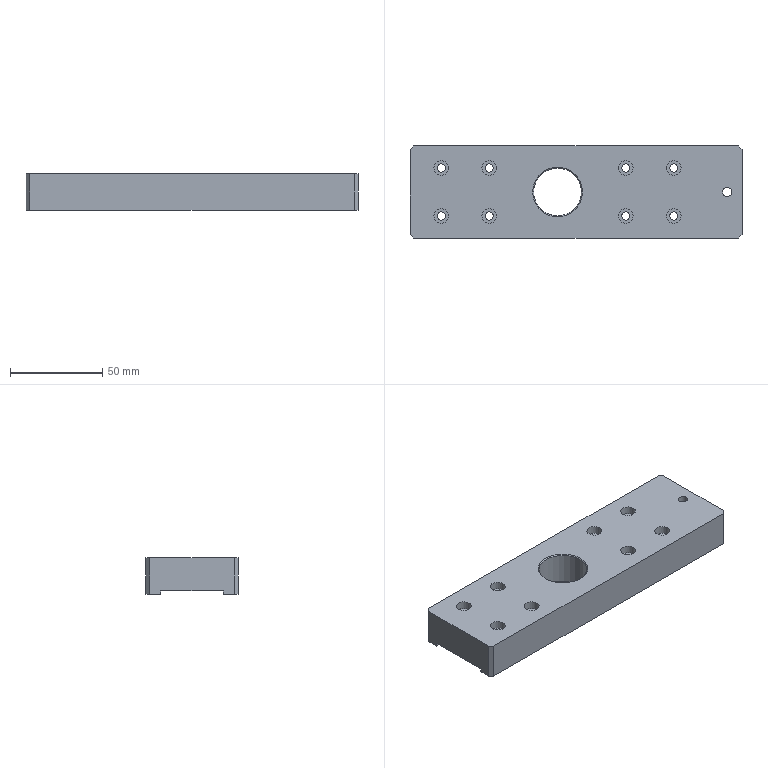Part | NX | 1 solid | 42 faces | box 180 x 50 x 20 mm | volume 154777 mm3 | plane 22 | cylinder 18 | cone 2 | commonest cylinder face diameters 4.5 x8 8 x8 5 x1 26 x1
STEP:
#1=CARTESIAN_POINT('',(-88.,25.,10.));
#2=VERTEX_POINT('',#1);
#3=CARTESIAN_POINT('',(-90.,23.,10.));
#4=VERTEX_POINT('',#3);
#5=CARTESIAN_POINT('',(-56.5,56.5,10.));
#6=DIRECTION('',(-0.7071,-0.7071,0.));
#7=VECTOR('',#6,1000.);
#8=LINE('',#5,#7);
#9=EDGE_CURVE('',#2,#4,#8,.T.);
#10=ORIENTED_EDGE('',*,*,#9,.F.);
#11=CARTESIAN_POINT('',(-88.,25.,-10.));
#12=VERTEX_POINT('',#11);
#13=CARTESIAN_POINT('',(-88.,25.,10.));
#14=DIRECTION('',(0.,0.,1.));
#15=VECTOR('',#14,1000.);
#16=LINE('',#13,#15);
#17=EDGE_CURVE('',#12,#2,#16,.T.);
#18=ORIENTED_EDGE('',*,*,#17,.F.);
#19=CARTESIAN_POINT('',(-90.,23.,-10.));
#20=VERTEX_POINT('',#19);
#21=CARTESIAN_POINT('',(-90.,23.,-10.));
#22=DIRECTION('',(0.7071,0.7071,0.));
#23=VECTOR('',#22,1000.);
#24=LINE('',#21,#23);
#25=EDGE_CURVE('',#20,#12,#24,.T.);
#26=ORIENTED_EDGE('',*,*,#25,.F.);
#27=CARTESIAN_POINT('',(-90.,23.,10.));
#28=DIRECTION('',(0.,0.,-1.));
#29=VECTOR('',#28,1000.);
#30=LINE('',#27,#29);
#31=EDGE_CURVE('',#4,#20,#30,.T.);
#32=ORIENTED_EDGE('',*,*,#31,.F.);
#33=EDGE_LOOP('',(#10,#18,#26,#32));
#34=FACE_BOUND('',#33,.T.);
#35=CARTESIAN_POINT('',(-90.,23.,10.));
#36=DIRECTION('',(0.7071,-0.7071,0.));
#37=DIRECTION('',(0.,0.,-1.));
#38=AXIS2_PLACEMENT_3D('',#35,#36,#37);
#39=PLANE('',#38);
#40=ADVANCED_FACE('',(#34),#39,.F.);
#41=CARTESIAN_POINT('',(-90.,-23.,10.));
#42=VERTEX_POINT('',#41);
#43=CARTESIAN_POINT('',(-88.,-25.,10.));
#44=VERTEX_POINT('',#43);
#45=CARTESIAN_POINT('',(-56.5,-56.5,10.));
#46=DIRECTION('',(0.7071,-0.7071,0.));
#47=VECTOR('',#46,1000.);
#48=LINE('',#45,#47);
#49=EDGE_CURVE('',#42,#44,#48,.T.);
#50=ORIENTED_EDGE('',*,*,#49,.F.);
#51=CARTESIAN_POINT('',(-90.,-23.,-10.));
#52=VERTEX_POINT('',#51);
#53=CARTESIAN_POINT('',(-90.,-23.,10.));
#54=DIRECTION('',(0.,0.,1.));
#55=VECTOR('',#54,1000.);
#56=LINE('',#53,#55);
#57=EDGE_CURVE('',#52,#42,#56,.T.);
#58=ORIENTED_EDGE('',*,*,#57,.F.);
#59=CARTESIAN_POINT('',(-88.,-25.,-10.));
#60=VERTEX_POINT('',#59);
#61=CARTESIAN_POINT('',(-88.,-25.,-10.));
#62=DIRECTION('',(-0.7071,0.7071,0.));
#63=VECTOR('',#62,1000.);
#64=LINE('',#61,#63);
#65=EDGE_CURVE('',#60,#52,#64,.T.);
#66=ORIENTED_EDGE('',*,*,#65,.F.);
#67=CARTESIAN_POINT('',(-88.,-25.,10.));
#68=DIRECTION('',(0.,0.,-1.));
#69=VECTOR('',#68,1000.);
#70=LINE('',#67,#69);
#71=EDGE_CURVE('',#44,#60,#70,.T.);
#72=ORIENTED_EDGE('',*,*,#71,.F.);
#73=EDGE_LOOP('',(#50,#58,#66,#72));
#74=FACE_BOUND('',#73,.T.);
#75=CARTESIAN_POINT('',(-88.,-25.,10.));
#76=DIRECTION('',(0.7071,0.7071,0.));
#77=DIRECTION('',(0.,0.,-1.));
#78=AXIS2_PLACEMENT_3D('',#75,#76,#77);
#79=PLANE('',#78);
#80=ADVANCED_FACE('',(#74),#79,.F.);
#81=CARTESIAN_POINT('',(88.,-25.,10.));
#82=VERTEX_POINT('',#81);
#83=CARTESIAN_POINT('',(90.,-23.,10.));
#84=VERTEX_POINT('',#83);
#85=CARTESIAN_POINT('',(56.5,-56.5,10.));
#86=DIRECTION('',(0.7071,0.7071,0.));
#87=VECTOR('',#86,1000.);
#88=LINE('',#85,#87);
#89=EDGE_CURVE('',#82,#84,#88,.T.);
#90=ORIENTED_EDGE('',*,*,#89,.F.);
#91=CARTESIAN_POINT('',(88.,-25.,-10.));
#92=VERTEX_POINT('',#91);
#93=CARTESIAN_POINT('',(88.,-25.,10.));
#94=DIRECTION('',(0.,0.,1.));
#95=VECTOR('',#94,1000.);
#96=LINE('',#93,#95);
#97=EDGE_CURVE('',#92,#82,#96,.T.);
#98=ORIENTED_EDGE('',*,*,#97,.F.);
#99=CARTESIAN_POINT('',(90.,-23.,-10.));
#100=VERTEX_POINT('',#99);
#101=CARTESIAN_POINT('',(90.,-23.,-10.));
#102=DIRECTION('',(-0.7071,-0.7071,0.));
#103=VECTOR('',#102,1000.);
#104=LINE('',#101,#103);
#105=EDGE_CURVE('',#100,#92,#104,.T.);
#106=ORIENTED_EDGE('',*,*,#105,.F.);
#107=CARTESIAN_POINT('',(90.,-23.,10.));
#108=DIRECTION('',(0.,0.,-1.));
#109=VECTOR('',#108,1000.);
#110=LINE('',#107,#109);
#111=EDGE_CURVE('',#84,#100,#110,.T.);
#112=ORIENTED_EDGE('',*,*,#111,.F.);
#113=EDGE_LOOP('',(#90,#98,#106,#112));
#114=FACE_BOUND('',#113,.T.);
#115=CARTESIAN_POINT('',(90.,-23.,10.));
#116=DIRECTION('',(-0.7071,0.7071,0.));
#117=DIRECTION('',(0.,0.,-1.));
#118=AXIS2_PLACEMENT_3D('',#115,#116,#117);
#119=PLANE('',#118);
#120=ADVANCED_FACE('',(#114),#119,.F.);
#121=CARTESIAN_POINT('',(90.,23.,10.));
#122=VERTEX_POINT('',#121);
#123=CARTESIAN_POINT('',(88.,25.,10.));
#124=VERTEX_POINT('',#123);
#125=CARTESIAN_POINT('',(56.5,56.5,10.));
#126=DIRECTION('',(-0.7071,0.7071,0.));
#127=VECTOR('',#126,1000.);
#128=LINE('',#125,#127);
#129=EDGE_CURVE('',#122,#124,#128,.T.);
#130=ORIENTED_EDGE('',*,*,#129,.F.);
#131=CARTESIAN_POINT('',(90.,23.,-10.));
#132=VERTEX_POINT('',#131);
#133=CARTESIAN_POINT('',(90.,23.,10.));
#134=DIRECTION('',(0.,0.,1.));
#135=VECTOR('',#134,1000.);
#136=LINE('',#133,#135);
#137=EDGE_CURVE('',#132,#122,#136,.T.);
#138=ORIENTED_EDGE('',*,*,#137,.F.);
#139=CARTESIAN_POINT('',(88.,25.,-10.));
#140=VERTEX_POINT('',#139);
#141=CARTESIAN_POINT('',(88.,25.,-10.));
#142=DIRECTION('',(0.7071,-0.7071,0.));
#143=VECTOR('',#142,1000.);
#144=LINE('',#141,#143);
#145=EDGE_CURVE('',#140,#132,#144,.T.);
#146=ORIENTED_EDGE('',*,*,#145,.F.);
#147=CARTESIAN_POINT('',(88.,25.,10.));
#148=DIRECTION('',(0.,0.,-1.));
#149=VECTOR('',#148,1000.);
#150=LINE('',#147,#149);
#151=EDGE_CURVE('',#124,#140,#150,.T.);
#152=ORIENTED_EDGE('',*,*,#151,.F.);
#153=EDGE_LOOP('',(#130,#138,#146,#152));
#154=FACE_BOUND('',#153,.T.);
#155=CARTESIAN_POINT('',(88.,25.,10.));
#156=DIRECTION('',(-0.7071,-0.7071,0.));
#157=DIRECTION('',(0.,0.,-1.));
#158=AXIS2_PLACEMENT_3D('',#155,#156,#157);
#159=PLANE('',#158);
#160=ADVANCED_FACE('',(#154),#159,.F.);
#161=CARTESIAN_POINT('',(-69.,13.,5.6));
#162=VERTEX_POINT('',#161);
#163=CARTESIAN_POINT('',(-73.,13.,5.6));
#164=DIRECTION('',(0.,0.,1.));
#165=DIRECTION('',(1.,0.,0.));
#166=AXIS2_PLACEMENT_3D('',#163,#164,#165);
#167=CIRCLE('',#166,4.);
#168=EDGE_CURVE('',#162,#162,#167,.T.);
#169=ORIENTED_EDGE('',*,*,#168,.T.);
#170=EDGE_LOOP('',(#169));
#171=FACE_BOUND('',#170,.T.);
#172=CARTESIAN_POINT('',(-70.75,13.,5.6));
#173=VERTEX_POINT('',#172);
#174=CARTESIAN_POINT('',(-73.,13.,5.6));
#175=DIRECTION('',(0.,0.,1.));
#176=DIRECTION('',(1.,0.,0.));
#177=AXIS2_PLACEMENT_3D('',#174,#175,#176);
#178=CIRCLE('',#177,2.25);
#179=EDGE_CURVE('',#173,#173,#178,.T.);
#180=ORIENTED_EDGE('',*,*,#179,.F.);
#181=EDGE_LOOP('',(#180));
#182=FACE_BOUND('',#181,.T.);
#183=CARTESIAN_POINT('',(-70.75,13.,5.6));
#184=DIRECTION('',(0.,0.,-1.));
#185=DIRECTION('',(-1.,0.,0.));
#186=AXIS2_PLACEMENT_3D('',#183,#184,#185);
#187=PLANE('',#186);
#188=ADVANCED_FACE('',(#171,#182),#187,.F.);
#189=CARTESIAN_POINT('',(-51.,13.,5.6));
#190=VERTEX_POINT('',#189);
#191=CARTESIAN_POINT('',(-47.,13.,5.6));
#192=DIRECTION('',(0.,0.,1.));
#193=DIRECTION('',(-1.,0.,0.));
#194=AXIS2_PLACEMENT_3D('',#191,#192,#193);
#195=CIRCLE('',#194,4.);
#196=EDGE_CURVE('',#190,#190,#195,.T.);
#197=ORIENTED_EDGE('',*,*,#196,.T.);
#198=EDGE_LOOP('',(#197));
#199=FACE_BOUND('',#198,.T.);
#200=CARTESIAN_POINT('',(-49.25,13.,5.6));
#201=VERTEX_POINT('',#200);
#202=CARTESIAN_POINT('',(-47.,13.,5.6));
#203=DIRECTION('',(0.,0.,1.));
#204=DIRECTION('',(-1.,0.,0.));
#205=AXIS2_PLACEMENT_3D('',#202,#203,#204);
#206=CIRCLE('',#205,2.25);
#207=EDGE_CURVE('',#201,#201,#206,.T.);
#208=ORIENTED_EDGE('',*,*,#207,.F.);
#209=EDGE_LOOP('',(#208));
#210=FACE_BOUND('',#209,.T.);
#211=CARTESIAN_POINT('',(-70.75,13.,5.6));
#212=DIRECTION('',(0.,0.,-1.));
#213=DIRECTION('',(-1.,0.,0.));
#214=AXIS2_PLACEMENT_3D('',#211,#212,#213);
#215=PLANE('',#214);
#216=ADVANCED_FACE('',(#199,#210),#215,.F.);
#217=CARTESIAN_POINT('',(-51.,-13.,5.6));
#218=VERTEX_POINT('',#217);
#219=CARTESIAN_POINT('',(-47.,-13.,5.6));
#220=DIRECTION('',(0.,0.,1.));
#221=DIRECTION('',(-1.,0.,0.));
#222=AXIS2_PLACEMENT_3D('',#219,#220,#221);
#223=CIRCLE('',#222,4.);
#224=EDGE_CURVE('',#218,#218,#223,.T.);
#225=ORIENTED_EDGE('',*,*,#224,.T.);
#226=EDGE_LOOP('',(#225));
#227=FACE_BOUND('',#226,.T.);
#228=CARTESIAN_POINT('',(-49.25,-13.,5.6));
#229=VERTEX_POINT('',#228);
#230=CARTESIAN_POINT('',(-47.,-13.,5.6));
#231=DIRECTION('',(0.,0.,1.));
#232=DIRECTION('',(-1.,0.,0.));
#233=AXIS2_PLACEMENT_3D('',#230,#231,#232);
#234=CIRCLE('',#233,2.25);
#235=EDGE_CURVE('',#229,#229,#234,.T.);
#236=ORIENTED_EDGE('',*,*,#235,.F.);
#237=EDGE_LOOP('',(#236));
#238=FACE_BOUND('',#237,.T.);
#239=CARTESIAN_POINT('',(-70.75,13.,5.6));
#240=DIRECTION('',(0.,0.,-1.));
#241=DIRECTION('',(-1.,0.,0.));
#242=AXIS2_PLACEMENT_3D('',#239,#240,#241);
#243=PLANE('',#242);
#244=ADVANCED_FACE('',(#227,#238),#243,.F.);
#245=CARTESIAN_POINT('',(-77.,-13.,5.6));
#246=VERTEX_POINT('',#245);
#247=CARTESIAN_POINT('',(-73.,-13.,5.6));
#248=DIRECTION('',(0.,0.,1.));
#249=DIRECTION('',(-1.,0.,0.));
#250=AXIS2_PLACEMENT_3D('',#247,#248,#249);
#251=CIRCLE('',#250,4.);
#252=EDGE_CURVE('',#246,#246,#251,.T.);
#253=ORIENTED_EDGE('',*,*,#252,.T.);
#254=EDGE_LOOP('',(#253));
#255=FACE_BOUND('',#254,.T.);
#256=CARTESIAN_POINT('',(-75.25,-13.,5.6));
#257=VERTEX_POINT('',#256);
#258=CARTESIAN_POINT('',(-73.,-13.,5.6));
#259=DIRECTION('',(0.,0.,1.));
#260=DIRECTION('',(-1.,0.,0.));
#261=AXIS2_PLACEMENT_3D('',#258,#259,#260);
#262=CIRCLE('',#261,2.25);
#263=EDGE_CURVE('',#257,#257,#262,.T.);
#264=ORIENTED_EDGE('',*,*,#263,.F.);
#265=EDGE_LOOP('',(#264));
#266=FACE_BOUND('',#265,.T.);
#267=CARTESIAN_POINT('',(-70.75,13.,5.6));
#268=DIRECTION('',(0.,0.,-1.));
#269=DIRECTION('',(-1.,0.,0.));
#270=AXIS2_PLACEMENT_3D('',#267,#268,#269);
#271=PLANE('',#270);
#272=ADVANCED_FACE('',(#255,#266),#271,.F.);
#273=CARTESIAN_POINT('',(23.,-13.,5.6));
#274=VERTEX_POINT('',#273);
#275=CARTESIAN_POINT('',(27.,-13.,5.6));
#276=DIRECTION('',(0.,0.,1.));
#277=DIRECTION('',(-1.,0.,0.));
#278=AXIS2_PLACEMENT_3D('',#275,#276,#277);
#279=CIRCLE('',#278,4.);
#280=EDGE_CURVE('',#274,#274,#279,.T.);
#281=ORIENTED_EDGE('',*,*,#280,.T.);
#282=EDGE_LOOP('',(#281));
#283=FACE_BOUND('',#282,.T.);
#284=CARTESIAN_POINT('',(24.75,-13.,5.6));
#285=VERTEX_POINT('',#284);
#286=CARTESIAN_POINT('',(27.,-13.,5.6));
#287=DIRECTION('',(0.,0.,1.));
#288=DIRECTION('',(-1.,0.,0.));
#289=AXIS2_PLACEMENT_3D('',#286,#287,#288);
#290=CIRCLE('',#289,2.25);
#291=EDGE_CURVE('',#285,#285,#290,.T.);
#292=ORIENTED_EDGE('',*,*,#291,.F.);
#293=EDGE_LOOP('',(#292));
#294=FACE_BOUND('',#293,.T.);
#295=CARTESIAN_POINT('',(-70.75,13.,5.6));
#296=DIRECTION('',(0.,0.,-1.));
#297=DIRECTION('',(-1.,0.,0.));
#298=AXIS2_PLACEMENT_3D('',#295,#296,#297);
#299=PLANE('',#298);
#300=ADVANCED_FACE('',(#283,#294),#299,.F.);
#301=CARTESIAN_POINT('',(23.,13.,5.6));
#302=VERTEX_POINT('',#301);
#303=CARTESIAN_POINT('',(27.,13.,5.6));
#304=DIRECTION('',(0.,0.,1.));
#305=DIRECTION('',(-1.,0.,0.));
#306=AXIS2_PLACEMENT_3D('',#303,#304,#305);
#307=CIRCLE('',#306,4.);
#308=EDGE_CURVE('',#302,#302,#307,.T.);
#309=ORIENTED_EDGE('',*,*,#308,.T.);
#310=EDGE_LOOP('',(#309));
#311=FACE_BOUND('',#310,.T.);
#312=CARTESIAN_POINT('',(24.75,13.,5.6));
#313=VERTEX_POINT('',#312);
#314=CARTESIAN_POINT('',(27.,13.,5.6));
#315=DIRECTION('',(0.,0.,1.));
#316=DIRECTION('',(-1.,0.,0.));
#317=AXIS2_PLACEMENT_3D('',#314,#315,#316);
#318=CIRCLE('',#317,2.25);
#319=EDGE_CURVE('',#313,#313,#318,.T.);
#320=ORIENTED_EDGE('',*,*,#319,.F.);
#321=EDGE_LOOP('',(#320));
#322=FACE_BOUND('',#321,.T.);
#323=CARTESIAN_POINT('',(-70.75,13.,5.6));
#324=DIRECTION('',(0.,0.,-1.));
#325=DIRECTION('',(-1.,0.,0.));
#326=AXIS2_PLACEMENT_3D('',#323,#324,#325);
#327=PLANE('',#326);
#328=ADVANCED_FACE('',(#311,#322),#327,.F.);
#329=CARTESIAN_POINT('',(49.,13.,5.6));
#330=VERTEX_POINT('',#329);
#331=CARTESIAN_POINT('',(53.,13.,5.6));
#332=DIRECTION('',(0.,0.,1.));
#333=DIRECTION('',(-1.,0.,0.));
#334=AXIS2_PLACEMENT_3D('',#331,#332,#333);
#335=CIRCLE('',#334,4.);
#336=EDGE_CURVE('',#330,#330,#335,.T.);
#337=ORIENTED_EDGE('',*,*,#336,.T.);
#338=EDGE_LOOP('',(#337));
#339=FACE_BOUND('',#338,.T.);
#340=CARTESIAN_POINT('',(50.75,13.,5.6));
#341=VERTEX_POINT('',#340);
#342=CARTESIAN_POINT('',(53.,13.,5.6));
#343=DIRECTION('',(0.,0.,1.));
#344=DIRECTION('',(-1.,0.,0.));
#345=AXIS2_PLACEMENT_3D('',#342,#343,#344);
#346=CIRCLE('',#345,2.25);
#347=EDGE_CURVE('',#341,#341,#346,.T.);
#348=ORIENTED_EDGE('',*,*,#347,.F.);
#349=EDGE_LOOP('',(#348));
#350=FACE_BOUND('',#349,.T.);
#351=CARTESIAN_POINT('',(-70.75,13.,5.6));
#352=DIRECTION('',(0.,0.,-1.));
#353=DIRECTION('',(-1.,0.,0.));
#354=AXIS2_PLACEMENT_3D('',#351,#352,#353);
#355=PLANE('',#354);
#356=ADVANCED_FACE('',(#339,#350),#355,.F.);
#357=CARTESIAN_POINT('',(49.,-13.,5.6));
#358=VERTEX_POINT('',#357);
#359=CARTESIAN_POINT('',(53.,-13.,5.6));
#360=DIRECTION('',(0.,0.,1.));
#361=DIRECTION('',(-1.,0.,0.));
#362=AXIS2_PLACEMENT_3D('',#359,#360,#361);
#363=CIRCLE('',#362,4.);
#364=EDGE_CURVE('',#358,#358,#363,.T.);
#365=ORIENTED_EDGE('',*,*,#364,.T.);
#366=EDGE_LOOP('',(#365));
#367=FACE_BOUND('',#366,.T.);
#368=CARTESIAN_POINT('',(50.75,-13.,5.6));
#369=VERTEX_POINT('',#368);
#370=CARTESIAN_POINT('',(53.,-13.,5.6));
#371=DIRECTION('',(0.,0.,1.));
#372=DIRECTION('',(-1.,0.,0.));
#373=AXIS2_PLACEMENT_3D('',#370,#371,#372);
#374=CIRCLE('',#373,2.25);
#375=EDGE_CURVE('',#369,#369,#374,.T.);
#376=ORIENTED_EDGE('',*,*,#375,.F.);
#377=EDGE_LOOP('',(#376));
#378=FACE_BOUND('',#377,.T.);
#379=CARTESIAN_POINT('',(-70.75,13.,5.6));
#380=DIRECTION('',(0.,0.,-1.));
#381=DIRECTION('',(-1.,0.,0.));
#382=AXIS2_PLACEMENT_3D('',#379,#380,#381);
#383=PLANE('',#382);
#384=ADVANCED_FACE('',(#367,#378),#383,.F.);
#385=CARTESIAN_POINT('',(90.,16.9,-8.1));
#386=VERTEX_POINT('',#385);
#387=CARTESIAN_POINT('',(90.,-16.9,-8.1));
#388=VERTEX_POINT('',#387);
#389=CARTESIAN_POINT('',(90.,0.,-8.1));
#390=DIRECTION('',(0.,-1.,0.));
#391=VECTOR('',#390,1000.);
#392=LINE('',#389,#391);
#393=EDGE_CURVE('',#386,#388,#392,.T.);
#394=ORIENTED_EDGE('',*,*,#393,.T.);
#395=CARTESIAN_POINT('',(-90.,-16.9,-8.1));
#396=VERTEX_POINT('',#395);
#397=CARTESIAN_POINT('',(0.,-16.9,-8.1));
#398=DIRECTION('',(-1.,0.,0.));
#399=VECTOR('',#398,1000.);
#400=LINE('',#397,#399);
#401=EDGE_CURVE('',#388,#396,#400,.T.);
#402=ORIENTED_EDGE('',*,*,#401,.T.);
#403=CARTESIAN_POINT('',(-90.,16.9,-8.1));
#404=VERTEX_POINT('',#403);
#405=CARTESIAN_POINT('',(-90.,0.,-8.1));
#406=DIRECTION('',(0.,1.,0.));
#407=VECTOR('',#406,1000.);
#408=LINE('',#405,#407);
#409=EDGE_CURVE('',#396,#404,#408,.T.);
#410=ORIENTED_EDGE('',*,*,#409,.T.);
#411=CARTESIAN_POINT('',(0.,16.9,-8.1));
#412=DIRECTION('',(1.,0.,0.));
#413=VECTOR('',#412,1000.);
#414=LINE('',#411,#413);
#415=EDGE_CURVE('',#404,#386,#414,.T.);
#416=ORIENTED_EDGE('',*,*,#415,.T.);
#417=EDGE_LOOP('',(#394,#402,#410,#416));
#418=FACE_BOUND('',#417,.T.);
#419=CARTESIAN_POINT('',(55.25,-13.,-8.1));
#420=VERTEX_POINT('',#419);
#421=CARTESIAN_POINT('',(53.,-13.,-8.1));
#422=DIRECTION('',(0.,0.,1.));
#423=DIRECTION('',(1.,0.,0.));
#424=AXIS2_PLACEMENT_3D('',#421,#422,#423);
#425=CIRCLE('',#424,2.25);
#426=EDGE_CURVE('',#420,#420,#425,.T.);
#427=ORIENTED_EDGE('',*,*,#426,.T.);
#428=EDGE_LOOP('',(#427));
#429=FACE_BOUND('',#428,.T.);
#430=CARTESIAN_POINT('',(55.25,13.,-8.1));
#431=VERTEX_POINT('',#430);
#432=CARTESIAN_POINT('',(53.,13.,-8.1));
#433=DIRECTION('',(0.,0.,1.));
#434=DIRECTION('',(1.,0.,0.));
#435=AXIS2_PLACEMENT_3D('',#432,#433,#434);
#436=CIRCLE('',#435,2.25);
#437=EDGE_CURVE('',#431,#431,#436,.T.);
#438=ORIENTED_EDGE('',*,*,#437,.T.);
#439=EDGE_LOOP('',(#438));
#440=FACE_BOUND('',#439,.T.);
#441=CARTESIAN_POINT('',(29.25,13.,-8.1));
#442=VERTEX_POINT('',#441);
#443=CARTESIAN_POINT('',(27.,13.,-8.1));
#444=DIRECTION('',(0.,0.,1.));
#445=DIRECTION('',(1.,0.,0.));
#446=AXIS2_PLACEMENT_3D('',#443,#444,#445);
#447=CIRCLE('',#446,2.25);
#448=EDGE_CURVE('',#442,#442,#447,.T.);
#449=ORIENTED_EDGE('',*,*,#448,.T.);
#450=EDGE_LOOP('',(#449));
#451=FACE_BOUND('',#450,.T.);
#452=CARTESIAN_POINT('',(29.25,-13.,-8.1));
#453=VERTEX_POINT('',#452);
#454=CARTESIAN_POINT('',(27.,-13.,-8.1));
#455=DIRECTION('',(0.,0.,1.));
#456=DIRECTION('',(1.,0.,0.));
#457=AXIS2_PLACEMENT_3D('',#454,#455,#456);
#458=CIRCLE('',#457,2.25);
#459=EDGE_CURVE('',#453,#453,#458,.T.);
#460=ORIENTED_EDGE('',*,*,#459,.T.);
#461=EDGE_LOOP('',(#460));
#462=FACE_BOUND('',#461,.T.);
#463=CARTESIAN_POINT('',(-70.75,-13.,-8.1));
#464=VERTEX_POINT('',#463);
#465=CARTESIAN_POINT('',(-73.,-13.,-8.1));
#466=DIRECTION('',(0.,0.,1.));
#467=DIRECTION('',(1.,0.,0.));
#468=AXIS2_PLACEMENT_3D('',#465,#466,#467);
#469=CIRCLE('',#468,2.25);
#470=EDGE_CURVE('',#464,#464,#469,.T.);
#471=ORIENTED_EDGE('',*,*,#470,.T.);
#472=EDGE_LOOP('',(#471));
#473=FACE_BOUND('',#472,.T.);
#474=CARTESIAN_POINT('',(-44.75,-13.,-8.1));
#475=VERTEX_POINT('',#474);
#476=CARTESIAN_POINT('',(-47.,-13.,-8.1));
#477=DIRECTION('',(0.,0.,1.));
#478=DIRECTION('',(1.,0.,0.));
#479=AXIS2_PLACEMENT_3D('',#476,#477,#478);
#480=CIRCLE('',#479,2.25);
#481=EDGE_CURVE('',#475,#475,#480,.T.);
#482=ORIENTED_EDGE('',*,*,#481,.T.);
#483=EDGE_LOOP('',(#482));
#484=FACE_BOUND('',#483,.T.);
#485=CARTESIAN_POINT('',(-44.75,13.,-8.1));
#486=VERTEX_POINT('',#485);
#487=CARTESIAN_POINT('',(-47.,13.,-8.1));
#488=DIRECTION('',(0.,0.,1.));
#489=DIRECTION('',(1.,0.,0.));
#490=AXIS2_PLACEMENT_3D('',#487,#488,#489);
#491=CIRCLE('',#490,2.25);
#492=EDGE_CURVE('',#486,#486,#491,.T.);
#493=ORIENTED_EDGE('',*,*,#492,.T.);
#494=EDGE_LOOP('',(#493));
#495=FACE_BOUND('',#494,.T.);
#496=CARTESIAN_POINT('',(-70.75,13.,-8.1));
#497=VERTEX_POINT('',#496);
#498=CARTESIAN_POINT('',(-73.,13.,-8.1));
#499=DIRECTION('',(0.,0.,1.));
#500=DIRECTION('',(1.,0.,0.));
#501=AXIS2_PLACEMENT_3D('',#498,#499,#500);
#502=CIRCLE('',#501,2.25);
#503=EDGE_CURVE('',#497,#497,#502,.T.);
#504=ORIENTED_EDGE('',*,*,#503,.T.);
#505=EDGE_LOOP('',(#504));
#506=FACE_BOUND('',#505,.T.);
#507=CARTESIAN_POINT('',(84.5,0.,-8.1));
#508=VERTEX_POINT('',#507);
#509=CARTESIAN_POINT('',(82.,0.,-8.1));
#510=DIRECTION('',(0.,0.,1.));
#511=DIRECTION('',(1.,0.,0.));
#512=AXIS2_PLACEMENT_3D('',#509,#510,#511);
#513=CIRCLE('',#512,2.5);
#514=EDGE_CURVE('',#508,#508,#513,.T.);
#515=ORIENTED_EDGE('',*,*,#514,.T.);
#516=EDGE_LOOP('',(#515));
#517=FACE_BOUND('',#516,.T.);
#518=CARTESIAN_POINT('',(3.6,0.,-8.1));
#519=VERTEX_POINT('',#518);
#520=CARTESIAN_POINT('',(-10.,0.,-8.1));
#521=DIRECTION('',(0.,0.,1.));
#522=DIRECTION('',(1.,0.,0.));
#523=AXIS2_PLACEMENT_3D('',#520,#521,#522);
#524=CIRCLE('',#523,13.6);
#525=EDGE_CURVE('',#519,#519,#524,.T.);
#526=ORIENTED_EDGE('',*,*,#525,.T.);
#527=EDGE_LOOP('',(#526));
#528=FACE_BOUND('',#527,.T.);
#529=CARTESIAN_POINT('',(0.,0.,-8.1));
#530=DIRECTION('',(0.,0.,1.));
#531=DIRECTION('',(1.,0.,0.));
#532=AXIS2_PLACEMENT_3D('',#529,#530,#531);
#533=PLANE('',#532);
#534=ADVANCED_FACE('',(#418,#429,#440,#451,#462,#473,#484,#495,#506,#517,#528),#533,.F.);
#535=CARTESIAN_POINT('',(-90.,16.9,-10.));
#536=VERTEX_POINT('',#535);
#537=CARTESIAN_POINT('',(90.,16.9,-10.));
#538=VERTEX_POINT('',#537);
#539=CARTESIAN_POINT('',(0.,16.9,-10.));
#540=DIRECTION('',(1.,0.,0.));
#541=VECTOR('',#540,1000.);
#542=LINE('',#539,#541);
#543=EDGE_CURVE('',#536,#538,#542,.T.);
#544=ORIENTED_EDGE('',*,*,#543,.T.);
#545=CARTESIAN_POINT('',(90.,16.9,10.));
#546=DIRECTION('',(0.,0.,1.));
#547=VECTOR('',#546,1000.);
#548=LINE('',#545,#547);
#549=EDGE_CURVE('',#538,#386,#548,.T.);
#550=ORIENTED_EDGE('',*,*,#549,.T.);
#551=ORIENTED_EDGE('',*,*,#415,.F.);
#552=CARTESIAN_POINT('',(-90.,16.9,-10.));
#553=DIRECTION('',(0.,0.,1.));
#554=VECTOR('',#553,1000.);
#555=LINE('',#552,#554);
#556=EDGE_CURVE('',#536,#404,#555,.T.);
#557=ORIENTED_EDGE('',*,*,#556,.F.);
#558=EDGE_LOOP('',(#544,#550,#551,#557));
#559=FACE_BOUND('',#558,.T.);
#560=CARTESIAN_POINT('',(90.,16.9,-10.));
#561=DIRECTION('',(0.,-1.,0.));
#562=DIRECTION('',(1.,0.,0.));
#563=AXIS2_PLACEMENT_3D('',#560,#561,#562);
#564=PLANE('',#563);
#565=ADVANCED_FACE('',(#559),#564,.T.);
#566=CARTESIAN_POINT('',(90.,-16.9,-10.));
#567=VERTEX_POINT('',#566);
#568=CARTESIAN_POINT('',(-90.,-16.9,-10.));
#569=VERTEX_POINT('',#568);
#570=CARTESIAN_POINT('',(0.,-16.9,-10.));
#571=DIRECTION('',(-1.,0.,0.));
#572=VECTOR('',#571,1000.);
#573=LINE('',#570,#572);
#574=EDGE_CURVE('',#567,#569,#573,.T.);
#575=ORIENTED_EDGE('',*,*,#574,.T.);
#576=CARTESIAN_POINT('',(-90.,-16.9,10.));
#577=DIRECTION('',(0.,0.,1.));
#578=VECTOR('',#577,1000.);
#579=LINE('',#576,#578);
#580=EDGE_CURVE('',#569,#396,#579,.T.);
#581=ORIENTED_EDGE('',*,*,#580,.T.);
#582=ORIENTED_EDGE('',*,*,#401,.F.);
#583=CARTESIAN_POINT('',(90.,-16.9,-10.));
#584=DIRECTION('',(0.,0.,1.));
#585=VECTOR('',#584,1000.);
#586=LINE('',#583,#585);
#587=EDGE_CURVE('',#567,#388,#586,.T.);
#588=ORIENTED_EDGE('',*,*,#587,.F.);
#589=EDGE_LOOP('',(#575,#581,#582,#588));
#590=FACE_BOUND('',#589,.T.);
#591=CARTESIAN_POINT('',(90.,-16.9,-10.));
#592=DIRECTION('',(0.,1.,0.));
#593=DIRECTION('',(-1.,0.,0.));
#594=AXIS2_PLACEMENT_3D('',#591,#592,#593);
#595=PLANE('',#594);
#596=ADVANCED_FACE('',(#590),#595,.T.);
#597=CARTESIAN_POINT('',(90.,-25.,10.));
#598=DIRECTION('',(0.,1.,0.));
#599=VECTOR('',#598,1000.);
#600=LINE('',#597,#599);
#601=EDGE_CURVE('',#84,#122,#600,.T.);
#602=ORIENTED_EDGE('',*,*,#601,.T.);
#603=ORIENTED_EDGE('',*,*,#129,.T.);
#604=CARTESIAN_POINT('',(90.,25.,10.));
#605=DIRECTION('',(-1.,0.,0.));
#606=VECTOR('',#605,1000.);
#607=LINE('',#604,#606);
#608=EDGE_CURVE('',#124,#2,#607,.T.);
#609=ORIENTED_EDGE('',*,*,#608,.T.);
#610=ORIENTED_EDGE('',*,*,#9,.T.);
#611=CARTESIAN_POINT('',(-90.,-25.,10.));
#612=DIRECTION('',(0.,-1.,0.));
#613=VECTOR('',#612,1000.);
#614=LINE('',#611,#613);
#615=EDGE_CURVE('',#4,#42,#614,.T.);
#616=ORIENTED_EDGE('',*,*,#615,.T.);
#617=ORIENTED_EDGE('',*,*,#49,.T.);
#618=CARTESIAN_POINT('',(90.,-25.,10.));
#619=DIRECTION('',(1.,0.,0.));
#620=VECTOR('',#619,1000.);
#621=LINE('',#618,#620);
#622=EDGE_CURVE('',#44,#82,#621,.T.);
#623=ORIENTED_EDGE('',*,*,#622,.T.);
#624=ORIENTED_EDGE('',*,*,#89,.T.);
#625=EDGE_LOOP('',(#602,#603,#609,#610,#616,#617,#623,#624));
#626=FACE_BOUND('',#625,.T.);
#627=CARTESIAN_POINT('',(57.,-13.,10.));
#628=VERTEX_POINT('',#627);
#629=CARTESIAN_POINT('',(53.,-13.,10.));
#630=DIRECTION('',(0.,0.,1.));
#631=DIRECTION('',(1.,0.,0.));
#632=AXIS2_PLACEMENT_3D('',#629,#630,#631);
#633=CIRCLE('',#632,4.);
#634=EDGE_CURVE('',#628,#628,#633,.T.);
#635=ORIENTED_EDGE('',*,*,#634,.F.);
#636=EDGE_LOOP('',(#635));
#637=FACE_BOUND('',#636,.T.);
#638=CARTESIAN_POINT('',(57.,13.,10.));
#639=VERTEX_POINT('',#638);
#640=CARTESIAN_POINT('',(53.,13.,10.));
#641=DIRECTION('',(0.,0.,1.));
#642=DIRECTION('',(1.,0.,0.));
#643=AXIS2_PLACEMENT_3D('',#640,#641,#642);
#644=CIRCLE('',#643,4.);
#645=EDGE_CURVE('',#639,#639,#644,.T.);
#646=ORIENTED_EDGE('',*,*,#645,.F.);
#647=EDGE_LOOP('',(#646));
#648=FACE_BOUND('',#647,.T.);
#649=CARTESIAN_POINT('',(31.,13.,10.));
#650=VERTEX_POINT('',#649);
#651=CARTESIAN_POINT('',(27.,13.,10.));
#652=DIRECTION('',(0.,0.,1.));
#653=DIRECTION('',(1.,0.,0.));
#654=AXIS2_PLACEMENT_3D('',#651,#652,#653);
#655=CIRCLE('',#654,4.);
#656=EDGE_CURVE('',#650,#650,#655,.T.);
#657=ORIENTED_EDGE('',*,*,#656,.F.);
#658=EDGE_LOOP('',(#657));
#659=FACE_BOUND('',#658,.T.);
#660=CARTESIAN_POINT('',(31.,-13.,10.));
#661=VERTEX_POINT('',#660);
#662=CARTESIAN_POINT('',(27.,-13.,10.));
#663=DIRECTION('',(0.,0.,1.));
#664=DIRECTION('',(1.,0.,0.));
#665=AXIS2_PLACEMENT_3D('',#662,#663,#664);
#666=CIRCLE('',#665,4.);
#667=EDGE_CURVE('',#661,#661,#666,.T.);
#668=ORIENTED_EDGE('',*,*,#667,.F.);
#669=EDGE_LOOP('',(#668));
#670=FACE_BOUND('',#669,.T.);
#671=CARTESIAN_POINT('',(-69.,-13.,10.));
#672=VERTEX_POINT('',#671);
#673=CARTESIAN_POINT('',(-73.,-13.,10.));
#674=DIRECTION('',(0.,0.,1.));
#675=DIRECTION('',(1.,0.,0.));
#676=AXIS2_PLACEMENT_3D('',#673,#674,#675);
#677=CIRCLE('',#676,4.);
#678=EDGE_CURVE('',#672,#672,#677,.T.);
#679=ORIENTED_EDGE('',*,*,#678,.F.);
#680=EDGE_LOOP('',(#679));
#681=FACE_BOUND('',#680,.T.);
#682=CARTESIAN_POINT('',(-43.,-13.,10.));
#683=VERTEX_POINT('',#682);
#684=CARTESIAN_POINT('',(-47.,-13.,10.));
#685=DIRECTION('',(0.,0.,1.));
#686=DIRECTION('',(1.,0.,0.));
#687=AXIS2_PLACEMENT_3D('',#684,#685,#686);
#688=CIRCLE('',#687,4.);
#689=EDGE_CURVE('',#683,#683,#688,.T.);
#690=ORIENTED_EDGE('',*,*,#689,.F.);
#691=EDGE_LOOP('',(#690));
#692=FACE_BOUND('',#691,.T.);
#693=CARTESIAN_POINT('',(-43.,13.,10.));
#694=VERTEX_POINT('',#693);
#695=CARTESIAN_POINT('',(-47.,13.,10.));
#696=DIRECTION('',(0.,0.,1.));
#697=DIRECTION('',(1.,0.,0.));
#698=AXIS2_PLACEMENT_3D('',#695,#696,#697);
#699=CIRCLE('',#698,4.);
#700=EDGE_CURVE('',#694,#694,#699,.T.);
#701=ORIENTED_EDGE('',*,*,#700,.F.);
#702=EDGE_LOOP('',(#701));
#703=FACE_BOUND('',#702,.T.);
#704=CARTESIAN_POINT('',(-69.,13.,10.));
#705=VERTEX_POINT('',#704);
#706=CARTESIAN_POINT('',(-73.,13.,10.));
#707=DIRECTION('',(0.,0.,1.));
#708=DIRECTION('',(1.,0.,0.));
#709=AXIS2_PLACEMENT_3D('',#706,#707,#708);
#710=CIRCLE('',#709,4.);
#711=EDGE_CURVE('',#705,#705,#710,.T.);
#712=ORIENTED_EDGE('',*,*,#711,.F.);
#713=EDGE_LOOP('',(#712));
#714=FACE_BOUND('',#713,.T.);
#715=CARTESIAN_POINT('',(84.5,0.,10.));
#716=VERTEX_POINT('',#715);
#717=CARTESIAN_POINT('',(82.,0.,10.));
#718=DIRECTION('',(0.,0.,1.));
#719=DIRECTION('',(1.,0.,0.));
#720=AXIS2_PLACEMENT_3D('',#717,#718,#719);
#721=CIRCLE('',#720,2.5);
#722=EDGE_CURVE('',#716,#716,#721,.T.);
#723=ORIENTED_EDGE('',*,*,#722,.F.);
#724=EDGE_LOOP('',(#723));
#725=FACE_BOUND('',#724,.T.);
#726=CARTESIAN_POINT('',(3.5,0.,10.));
#727=VERTEX_POINT('',#726);
#728=CARTESIAN_POINT('',(-10.,0.,10.));
#729=DIRECTION('',(0.,0.,-1.));
#730=DIRECTION('',(1.,0.,0.));
#731=AXIS2_PLACEMENT_3D('',#728,#729,#730);
#732=CIRCLE('',#731,13.5);
#733=EDGE_CURVE('',#727,#727,#732,.T.);
#734=ORIENTED_EDGE('',*,*,#733,.T.);
#735=EDGE_LOOP('',(#734));
#736=FACE_BOUND('',#735,.T.);
#737=CARTESIAN_POINT('',(0.,0.,10.));
#738=DIRECTION('',(0.,0.,1.));
#739=DIRECTION('',(1.,0.,0.));
#740=AXIS2_PLACEMENT_3D('',#737,#738,#739);
#741=PLANE('',#740);
#742=ADVANCED_FACE('',(#626,#637,#648,#659,#670,#681,#692,#703,#714,#725,#736),#741,.T.);
#743=ORIENTED_EDGE('',*,*,#608,.F.);
#744=ORIENTED_EDGE('',*,*,#151,.T.);
#745=CARTESIAN_POINT('',(90.,25.,-10.));
#746=DIRECTION('',(-1.,0.,0.));
#747=VECTOR('',#746,1000.);
#748=LINE('',#745,#747);
#749=EDGE_CURVE('',#140,#12,#748,.T.);
#750=ORIENTED_EDGE('',*,*,#749,.T.);
#751=ORIENTED_EDGE('',*,*,#17,.T.);
#752=EDGE_LOOP('',(#743,#744,#750,#751));
#753=FACE_BOUND('',#752,.T.);
#754=CARTESIAN_POINT('',(90.,25.,10.));
#755=DIRECTION('',(0.,-1.,0.));
#756=DIRECTION('',(1.,0.,0.));
#757=AXIS2_PLACEMENT_3D('',#754,#755,#756);
#758=PLANE('',#757);
#759=ADVANCED_FACE('',(#753),#758,.F.);
#760=CARTESIAN_POINT('',(90.,-25.,-10.));
#761=DIRECTION('',(1.,0.,0.));
#762=VECTOR('',#761,1000.);
#763=LINE('',#760,#762);
#764=EDGE_CURVE('',#60,#92,#763,.T.);
#765=ORIENTED_EDGE('',*,*,#764,.T.);
#766=ORIENTED_EDGE('',*,*,#97,.T.);
#767=ORIENTED_EDGE('',*,*,#622,.F.);
#768=ORIENTED_EDGE('',*,*,#71,.T.);
#769=EDGE_LOOP('',(#765,#766,#767,#768));
#770=FACE_BOUND('',#769,.T.);
#771=CARTESIAN_POINT('',(90.,-25.,10.));
#772=DIRECTION('',(0.,1.,0.));
#773=DIRECTION('',(-1.,0.,0.));
#774=AXIS2_PLACEMENT_3D('',#771,#772,#773);
#775=PLANE('',#774);
#776=ADVANCED_FACE('',(#770),#775,.F.);
#777=ORIENTED_EDGE('',*,*,#749,.F.);
#778=ORIENTED_EDGE('',*,*,#145,.T.);
#779=CARTESIAN_POINT('',(90.,-25.,-10.));
#780=DIRECTION('',(0.,1.,0.));
#781=VECTOR('',#780,1000.);
#782=LINE('',#779,#781);
#783=EDGE_CURVE('',#538,#132,#782,.T.);
#784=ORIENTED_EDGE('',*,*,#783,.F.);
#785=ORIENTED_EDGE('',*,*,#543,.F.);
#786=CARTESIAN_POINT('',(-90.,-25.,-10.));
#787=DIRECTION('',(0.,-1.,0.));
#788=VECTOR('',#787,1000.);
#789=LINE('',#786,#788);
#790=EDGE_CURVE('',#20,#536,#789,.T.);
#791=ORIENTED_EDGE('',*,*,#790,.F.);
#792=ORIENTED_EDGE('',*,*,#25,.T.);
#793=EDGE_LOOP('',(#777,#778,#784,#785,#791,#792));
#794=FACE_BOUND('',#793,.T.);
#795=CARTESIAN_POINT('',(0.,0.,-10.));
#796=DIRECTION('',(0.,0.,1.));
#797=DIRECTION('',(1.,0.,0.));
#798=AXIS2_PLACEMENT_3D('',#795,#796,#797);
#799=PLANE('',#798);
#800=ADVANCED_FACE('',(#794),#799,.F.);
#801=CARTESIAN_POINT('',(90.,-25.,-10.));
#802=DIRECTION('',(0.,1.,0.));
#803=VECTOR('',#802,1000.);
#804=LINE('',#801,#803);
#805=EDGE_CURVE('',#100,#567,#804,.T.);
#806=ORIENTED_EDGE('',*,*,#805,.F.);
#807=ORIENTED_EDGE('',*,*,#105,.T.);
#808=ORIENTED_EDGE('',*,*,#764,.F.);
#809=ORIENTED_EDGE('',*,*,#65,.T.);
#810=CARTESIAN_POINT('',(-90.,-25.,-10.));
#811=DIRECTION('',(0.,-1.,0.));
#812=VECTOR('',#811,1000.);
#813=LINE('',#810,#812);
#814=EDGE_CURVE('',#569,#52,#813,.T.);
#815=ORIENTED_EDGE('',*,*,#814,.F.);
#816=ORIENTED_EDGE('',*,*,#574,.F.);
#817=EDGE_LOOP('',(#806,#807,#808,#809,#815,#816));
#818=FACE_BOUND('',#817,.T.);
#819=CARTESIAN_POINT('',(0.,0.,-10.));
#820=DIRECTION('',(0.,0.,1.));
#821=DIRECTION('',(1.,0.,0.));
#822=AXIS2_PLACEMENT_3D('',#819,#820,#821);
#823=PLANE('',#822);
#824=ADVANCED_FACE('',(#818),#823,.F.);
#825=ORIENTED_EDGE('',*,*,#783,.T.);
#826=ORIENTED_EDGE('',*,*,#137,.T.);
#827=ORIENTED_EDGE('',*,*,#601,.F.);
#828=ORIENTED_EDGE('',*,*,#111,.T.);
#829=ORIENTED_EDGE('',*,*,#805,.T.);
#830=ORIENTED_EDGE('',*,*,#587,.T.);
#831=ORIENTED_EDGE('',*,*,#393,.F.);
#832=ORIENTED_EDGE('',*,*,#549,.F.);
#833=EDGE_LOOP('',(#825,#826,#827,#828,#829,#830,#831,#832));
#834=FACE_BOUND('',#833,.T.);
#835=CARTESIAN_POINT('',(90.,-25.,10.));
#836=DIRECTION('',(-1.,0.,0.));
#837=DIRECTION('',(0.,0.,1.));
#838=AXIS2_PLACEMENT_3D('',#835,#836,#837);
#839=PLANE('',#838);
#840=ADVANCED_FACE('',(#834),#839,.F.);
#841=ORIENTED_EDGE('',*,*,#814,.T.);
#842=ORIENTED_EDGE('',*,*,#57,.T.);
#843=ORIENTED_EDGE('',*,*,#615,.F.);
#844=ORIENTED_EDGE('',*,*,#31,.T.);
#845=ORIENTED_EDGE('',*,*,#790,.T.);
#846=ORIENTED_EDGE('',*,*,#556,.T.);
#847=ORIENTED_EDGE('',*,*,#409,.F.);
#848=ORIENTED_EDGE('',*,*,#580,.F.);
#849=EDGE_LOOP('',(#841,#842,#843,#844,#845,#846,#847,#848));
#850=FACE_BOUND('',#849,.T.);
#851=CARTESIAN_POINT('',(-90.,-25.,10.));
#852=DIRECTION('',(1.,0.,0.));
#853=DIRECTION('',(0.,0.,-1.));
#854=AXIS2_PLACEMENT_3D('',#851,#852,#853);
#855=PLANE('',#854);
#856=ADVANCED_FACE('',(#850),#855,.F.);
#857=CARTESIAN_POINT('',(3.,0.,-7.5));
#858=VERTEX_POINT('',#857);
#859=CARTESIAN_POINT('',(-10.,0.,-7.5));
#860=DIRECTION('',(0.,0.,-1.));
#861=DIRECTION('',(1.,0.,0.));
#862=AXIS2_PLACEMENT_3D('',#859,#860,#861);
#863=CIRCLE('',#862,13.);
#864=EDGE_CURVE('',#858,#858,#863,.T.);
#865=ORIENTED_EDGE('',*,*,#864,.T.);
#866=EDGE_LOOP('',(#865));
#867=FACE_BOUND('',#866,.T.);
#868=CARTESIAN_POINT('',(3.,0.,9.5));
#869=VERTEX_POINT('',#868);
#870=CARTESIAN_POINT('',(-10.,0.,9.5));
#871=DIRECTION('',(0.,0.,1.));
#872=DIRECTION('',(1.,0.,0.));
#873=AXIS2_PLACEMENT_3D('',#870,#871,#872);
#874=CIRCLE('',#873,13.);
#875=EDGE_CURVE('',#869,#869,#874,.T.);
#876=ORIENTED_EDGE('',*,*,#875,.T.);
#877=EDGE_LOOP('',(#876));
#878=FACE_BOUND('',#877,.T.);
#879=CARTESIAN_POINT('',(-10.,0.,-10.));
#880=DIRECTION('',(0.,0.,1.));
#881=DIRECTION('',(1.,0.,0.));
#882=AXIS2_PLACEMENT_3D('',#879,#880,#881);
#883=CYLINDRICAL_SURFACE('',#882,13.);
#884=ADVANCED_FACE('',(#867,#878),#883,.F.);
#885=ORIENTED_EDGE('',*,*,#426,.F.);
#886=EDGE_LOOP('',(#885));
#887=FACE_BOUND('',#886,.T.);
#888=ORIENTED_EDGE('',*,*,#375,.T.);
#889=EDGE_LOOP('',(#888));
#890=FACE_BOUND('',#889,.T.);
#891=CARTESIAN_POINT('',(53.,-13.,10.));
#892=DIRECTION('',(0.,0.,1.));
#893=DIRECTION('',(1.,0.,0.));
#894=AXIS2_PLACEMENT_3D('',#891,#892,#893);
#895=CYLINDRICAL_SURFACE('',#894,2.25);
#896=ADVANCED_FACE('',(#887,#890),#895,.F.);
#897=ORIENTED_EDGE('',*,*,#364,.F.);
#898=EDGE_LOOP('',(#897));
#899=FACE_BOUND('',#898,.T.);
#900=ORIENTED_EDGE('',*,*,#634,.T.);
#901=EDGE_LOOP('',(#900));
#902=FACE_BOUND('',#901,.T.);
#903=CARTESIAN_POINT('',(53.,-13.,10.));
#904=DIRECTION('',(0.,0.,1.));
#905=DIRECTION('',(1.,0.,0.));
#906=AXIS2_PLACEMENT_3D('',#903,#904,#905);
#907=CYLINDRICAL_SURFACE('',#906,4.);
#908=ADVANCED_FACE('',(#899,#902),#907,.F.);
#909=ORIENTED_EDGE('',*,*,#437,.F.);
#910=EDGE_LOOP('',(#909));
#911=FACE_BOUND('',#910,.T.);
#912=ORIENTED_EDGE('',*,*,#347,.T.);
#913=EDGE_LOOP('',(#912));
#914=FACE_BOUND('',#913,.T.);
#915=CARTESIAN_POINT('',(53.,13.,10.));
#916=DIRECTION('',(0.,0.,1.));
#917=DIRECTION('',(1.,0.,0.));
#918=AXIS2_PLACEMENT_3D('',#915,#916,#917);
#919=CYLINDRICAL_SURFACE('',#918,2.25);
#920=ADVANCED_FACE('',(#911,#914),#919,.F.);
#921=ORIENTED_EDGE('',*,*,#336,.F.);
#922=EDGE_LOOP('',(#921));
#923=FACE_BOUND('',#922,.T.);
#924=ORIENTED_EDGE('',*,*,#645,.T.);
#925=EDGE_LOOP('',(#924));
#926=FACE_BOUND('',#925,.T.);
#927=CARTESIAN_POINT('',(53.,13.,10.));
#928=DIRECTION('',(0.,0.,1.));
#929=DIRECTION('',(1.,0.,0.));
#930=AXIS2_PLACEMENT_3D('',#927,#928,#929);
#931=CYLINDRICAL_SURFACE('',#930,4.);
#932=ADVANCED_FACE('',(#923,#926),#931,.F.);
#933=ORIENTED_EDGE('',*,*,#448,.F.);
#934=EDGE_LOOP('',(#933));
#935=FACE_BOUND('',#934,.T.);
#936=ORIENTED_EDGE('',*,*,#319,.T.);
#937=EDGE_LOOP('',(#936));
#938=FACE_BOUND('',#937,.T.);
#939=CARTESIAN_POINT('',(27.,13.,10.));
#940=DIRECTION('',(0.,0.,1.));
#941=DIRECTION('',(1.,0.,0.));
#942=AXIS2_PLACEMENT_3D('',#939,#940,#941);
#943=CYLINDRICAL_SURFACE('',#942,2.25);
#944=ADVANCED_FACE('',(#935,#938),#943,.F.);
#945=ORIENTED_EDGE('',*,*,#308,.F.);
#946=EDGE_LOOP('',(#945));
#947=FACE_BOUND('',#946,.T.);
#948=ORIENTED_EDGE('',*,*,#656,.T.);
#949=EDGE_LOOP('',(#948));
#950=FACE_BOUND('',#949,.T.);
#951=CARTESIAN_POINT('',(27.,13.,10.));
#952=DIRECTION('',(0.,0.,1.));
#953=DIRECTION('',(1.,0.,0.));
#954=AXIS2_PLACEMENT_3D('',#951,#952,#953);
#955=CYLINDRICAL_SURFACE('',#954,4.);
#956=ADVANCED_FACE('',(#947,#950),#955,.F.);
#957=ORIENTED_EDGE('',*,*,#459,.F.);
#958=EDGE_LOOP('',(#957));
#959=FACE_BOUND('',#958,.T.);
#960=ORIENTED_EDGE('',*,*,#291,.T.);
#961=EDGE_LOOP('',(#960));
#962=FACE_BOUND('',#961,.T.);
#963=CARTESIAN_POINT('',(27.,-13.,10.));
#964=DIRECTION('',(0.,0.,1.));
#965=DIRECTION('',(1.,0.,0.));
#966=AXIS2_PLACEMENT_3D('',#963,#964,#965);
#967=CYLINDRICAL_SURFACE('',#966,2.25);
#968=ADVANCED_FACE('',(#959,#962),#967,.F.);
#969=ORIENTED_EDGE('',*,*,#280,.F.);
#970=EDGE_LOOP('',(#969));
#971=FACE_BOUND('',#970,.T.);
#972=ORIENTED_EDGE('',*,*,#667,.T.);
#973=EDGE_LOOP('',(#972));
#974=FACE_BOUND('',#973,.T.);
#975=CARTESIAN_POINT('',(27.,-13.,10.));
#976=DIRECTION('',(0.,0.,1.));
#977=DIRECTION('',(1.,0.,0.));
#978=AXIS2_PLACEMENT_3D('',#975,#976,#977);
#979=CYLINDRICAL_SURFACE('',#978,4.);
#980=ADVANCED_FACE('',(#971,#974),#979,.F.);
#981=ORIENTED_EDGE('',*,*,#470,.F.);
#982=EDGE_LOOP('',(#981));
#983=FACE_BOUND('',#982,.T.);
#984=ORIENTED_EDGE('',*,*,#263,.T.);
#985=EDGE_LOOP('',(#984));
#986=FACE_BOUND('',#985,.T.);
#987=CARTESIAN_POINT('',(-73.,-13.,10.));
#988=DIRECTION('',(0.,0.,1.));
#989=DIRECTION('',(1.,0.,0.));
#990=AXIS2_PLACEMENT_3D('',#987,#988,#989);
#991=CYLINDRICAL_SURFACE('',#990,2.25);
#992=ADVANCED_FACE('',(#983,#986),#991,.F.);
#993=ORIENTED_EDGE('',*,*,#252,.F.);
#994=EDGE_LOOP('',(#993));
#995=FACE_BOUND('',#994,.T.);
#996=ORIENTED_EDGE('',*,*,#678,.T.);
#997=EDGE_LOOP('',(#996));
#998=FACE_BOUND('',#997,.T.);
#999=CARTESIAN_POINT('',(-73.,-13.,10.));
#1000=DIRECTION('',(0.,0.,1.));
#1001=DIRECTION('',(1.,0.,0.));
#1002=AXIS2_PLACEMENT_3D('',#999,#1000,#1001);
#1003=CYLINDRICAL_SURFACE('',#1002,4.);
#1004=ADVANCED_FACE('',(#995,#998),#1003,.F.);
#1005=ORIENTED_EDGE('',*,*,#481,.F.);
#1006=EDGE_LOOP('',(#1005));
#1007=FACE_BOUND('',#1006,.T.);
#1008=ORIENTED_EDGE('',*,*,#235,.T.);
#1009=EDGE_LOOP('',(#1008));
#1010=FACE_BOUND('',#1009,.T.);
#1011=CARTESIAN_POINT('',(-47.,-13.,10.));
#1012=DIRECTION('',(0.,0.,1.));
#1013=DIRECTION('',(1.,0.,0.));
#1014=AXIS2_PLACEMENT_3D('',#1011,#1012,#1013);
#1015=CYLINDRICAL_SURFACE('',#1014,2.25);
#1016=ADVANCED_FACE('',(#1007,#1010),#1015,.F.);
#1017=ORIENTED_EDGE('',*,*,#224,.F.);
#1018=EDGE_LOOP('',(#1017));
#1019=FACE_BOUND('',#1018,.T.);
#1020=ORIENTED_EDGE('',*,*,#689,.T.);
#1021=EDGE_LOOP('',(#1020));
#1022=FACE_BOUND('',#1021,.T.);
#1023=CARTESIAN_POINT('',(-47.,-13.,10.));
#1024=DIRECTION('',(0.,0.,1.));
#1025=DIRECTION('',(1.,0.,0.));
#1026=AXIS2_PLACEMENT_3D('',#1023,#1024,#1025);
#1027=CYLINDRICAL_SURFACE('',#1026,4.);
#1028=ADVANCED_FACE('',(#1019,#1022),#1027,.F.);
#1029=ORIENTED_EDGE('',*,*,#492,.F.);
#1030=EDGE_LOOP('',(#1029));
#1031=FACE_BOUND('',#1030,.T.);
#1032=ORIENTED_EDGE('',*,*,#207,.T.);
#1033=EDGE_LOOP('',(#1032));
#1034=FACE_BOUND('',#1033,.T.);
#1035=CARTESIAN_POINT('',(-47.,13.,10.));
#1036=DIRECTION('',(0.,0.,1.));
#1037=DIRECTION('',(1.,0.,0.));
#1038=AXIS2_PLACEMENT_3D('',#1035,#1036,#1037);
#1039=CYLINDRICAL_SURFACE('',#1038,2.25);
#1040=ADVANCED_FACE('',(#1031,#1034),#1039,.F.);
#1041=ORIENTED_EDGE('',*,*,#196,.F.);
#1042=EDGE_LOOP('',(#1041));
#1043=FACE_BOUND('',#1042,.T.);
#1044=ORIENTED_EDGE('',*,*,#700,.T.);
#1045=EDGE_LOOP('',(#1044));
#1046=FACE_BOUND('',#1045,.T.);
#1047=CARTESIAN_POINT('',(-47.,13.,10.));
#1048=DIRECTION('',(0.,0.,1.));
#1049=DIRECTION('',(1.,0.,0.));
#1050=AXIS2_PLACEMENT_3D('',#1047,#1048,#1049);
#1051=CYLINDRICAL_SURFACE('',#1050,4.);
#1052=ADVANCED_FACE('',(#1043,#1046),#1051,.F.);
#1053=ORIENTED_EDGE('',*,*,#503,.F.);
#1054=EDGE_LOOP('',(#1053));
#1055=FACE_BOUND('',#1054,.T.);
#1056=ORIENTED_EDGE('',*,*,#179,.T.);
#1057=EDGE_LOOP('',(#1056));
#1058=FACE_BOUND('',#1057,.T.);
#1059=CARTESIAN_POINT('',(-73.,13.,10.));
#1060=DIRECTION('',(0.,0.,1.));
#1061=DIRECTION('',(1.,0.,0.));
#1062=AXIS2_PLACEMENT_3D('',#1059,#1060,#1061);
#1063=CYLINDRICAL_SURFACE('',#1062,2.25);
#1064=ADVANCED_FACE('',(#1055,#1058),#1063,.F.);
#1065=ORIENTED_EDGE('',*,*,#168,.F.);
#1066=EDGE_LOOP('',(#1065));
#1067=FACE_BOUND('',#1066,.T.);
#1068=ORIENTED_EDGE('',*,*,#711,.T.);
#1069=EDGE_LOOP('',(#1068));
#1070=FACE_BOUND('',#1069,.T.);
#1071=CARTESIAN_POINT('',(-73.,13.,10.));
#1072=DIRECTION('',(0.,0.,1.));
#1073=DIRECTION('',(1.,0.,0.));
#1074=AXIS2_PLACEMENT_3D('',#1071,#1072,#1073);
#1075=CYLINDRICAL_SURFACE('',#1074,4.);
#1076=ADVANCED_FACE('',(#1067,#1070),#1075,.F.);
#1077=ORIENTED_EDGE('',*,*,#514,.F.);
#1078=EDGE_LOOP('',(#1077));
#1079=FACE_BOUND('',#1078,.T.);
#1080=ORIENTED_EDGE('',*,*,#722,.T.);
#1081=EDGE_LOOP('',(#1080));
#1082=FACE_BOUND('',#1081,.T.);
#1083=CARTESIAN_POINT('',(82.,0.,10.));
#1084=DIRECTION('',(0.,0.,1.));
#1085=DIRECTION('',(1.,0.,0.));
#1086=AXIS2_PLACEMENT_3D('',#1083,#1084,#1085);
#1087=CYLINDRICAL_SURFACE('',#1086,2.5);
#1088=ADVANCED_FACE('',(#1079,#1082),#1087,.F.);
#1089=ORIENTED_EDGE('',*,*,#525,.F.);
#1090=EDGE_LOOP('',(#1089));
#1091=FACE_BOUND('',#1090,.T.);
#1092=ORIENTED_EDGE('',*,*,#864,.F.);
#1093=EDGE_LOOP('',(#1092));
#1094=FACE_BOUND('',#1093,.T.);
#1095=CARTESIAN_POINT('',(-10.,0.,-7.5));
#1096=DIRECTION('',(0.,0.,-1.));
#1097=DIRECTION('',(-1.,0.,0.));
#1098=AXIS2_PLACEMENT_3D('',#1095,#1096,#1097);
#1099=CONICAL_SURFACE('',#1098,13.,0.7854);
#1100=ADVANCED_FACE('',(#1091,#1094),#1099,.F.);
#1101=ORIENTED_EDGE('',*,*,#875,.F.);
#1102=EDGE_LOOP('',(#1101));
#1103=FACE_BOUND('',#1102,.T.);
#1104=ORIENTED_EDGE('',*,*,#733,.F.);
#1105=EDGE_LOOP('',(#1104));
#1106=FACE_BOUND('',#1105,.T.);
#1107=CARTESIAN_POINT('',(-10.,0.,9.5));
#1108=DIRECTION('',(0.,0.,1.));
#1109=DIRECTION('',(1.,0.,0.));
#1110=AXIS2_PLACEMENT_3D('',#1107,#1108,#1109);
#1111=CONICAL_SURFACE('',#1110,13.,0.7854);
#1112=ADVANCED_FACE('',(#1103,#1106),#1111,.F.);
#1113=CLOSED_SHELL('',(#40,#80,#120,#160,#188,#216,#244,#272,#300,#328,#356,#384,#534,#565,#596,#742,#759,#776,#800,#824,#840,#856,#884,#896,#908,#920,#932,#944,#956,#968,#980,#992,#1004,#1016,#1028,#1040,#1052,#1064,#1076,#1088,#1100,#1112));
#1114=MANIFOLD_SOLID_BREP('',#1113);
#1115=(LENGTH_UNIT()NAMED_UNIT(*)SI_UNIT(.MILLI.,.METRE.));
#1116=UNCERTAINTY_MEASURE_WITH_UNIT(LENGTH_MEASURE(0.00001),#1115,'','');
#1117=(NAMED_UNIT(*)PLANE_ANGLE_UNIT()SI_UNIT($,.RADIAN.));
#1118=(NAMED_UNIT(*)SI_UNIT($,.STERADIAN.)SOLID_ANGLE_UNIT());
#1119=(GEOMETRIC_REPRESENTATION_CONTEXT(3)GLOBAL_UNCERTAINTY_ASSIGNED_CONTEXT((#1116))GLOBAL_UNIT_ASSIGNED_CONTEXT((#1115,#1117,#1118))REPRESENTATION_CONTEXT('',''));
#1120=ADVANCED_BREP_SHAPE_REPRESENTATION('',(#1114),#1119);